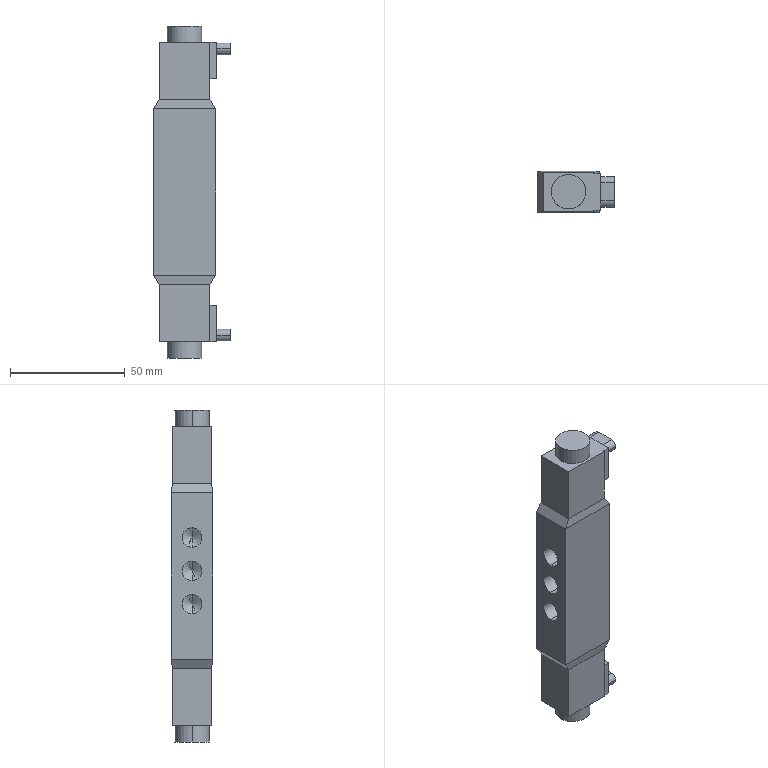Part | STEP file | double solenoid valve 4V120-06 | 1 solid | 68 faces | box 33.5 x 18 x 144.5 mm | volume 59015 mm3 | plane 38 | cylinder 20 | cone 10 | commonest cylinder face diameters 8.5 x10 5 x6 15 x4